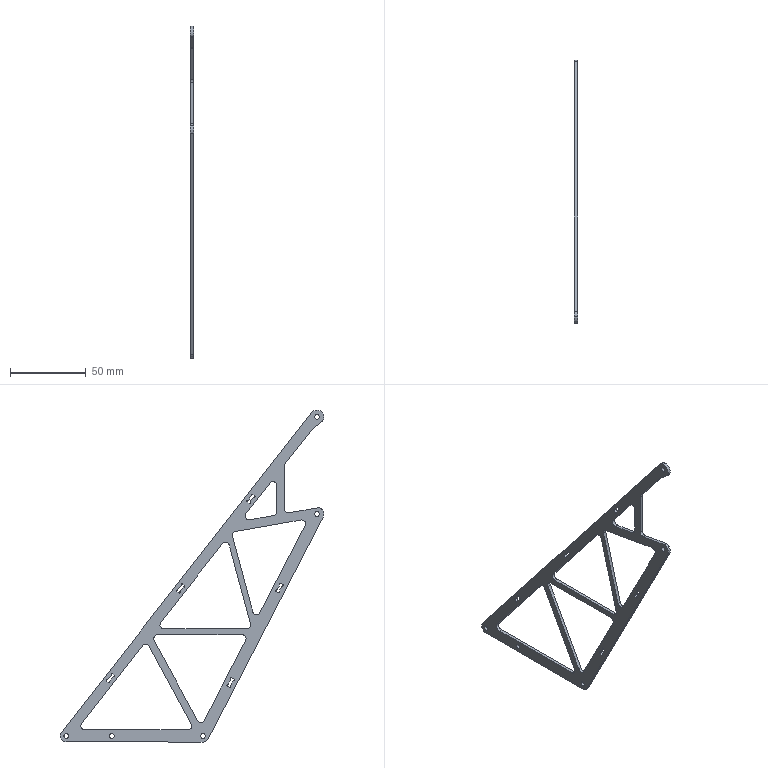Part | SolidWorks | features ICE 2, Extrusion 1, Fillet 1 | 1 solid | 110 faces | box 2 x 173.5 x 218.5 mm | volume 10390 mm3 | cylinder 66 | plane 44 | commonest cylinder face diameters 5 x21 1.05 x18 1.2 x12 3.1 x10 9 x3 8 x2